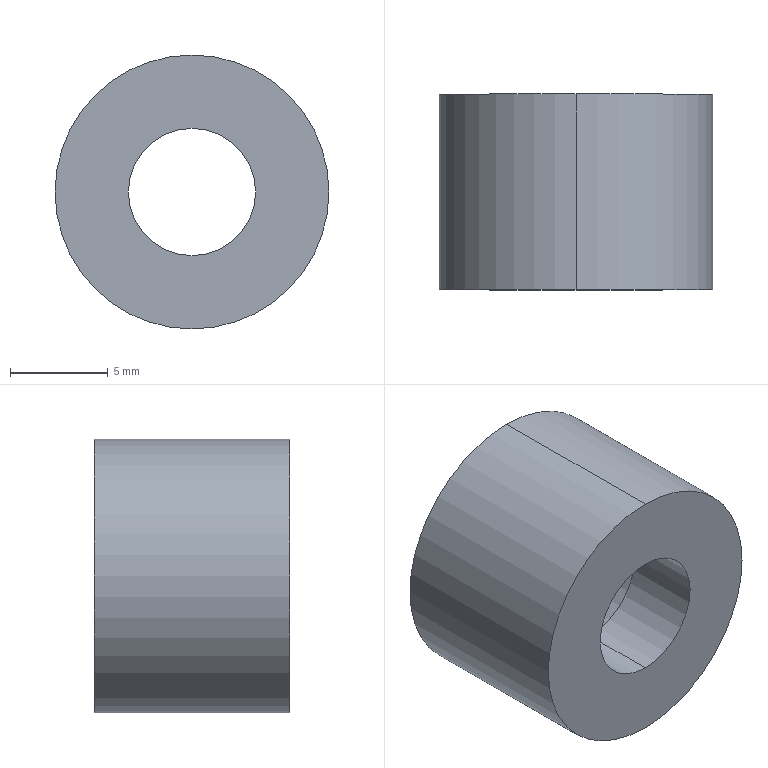Part | STEP file | OP10-160_seal pad (2nd air pass) | 1 solid | 9 faces | box 14 x 10 x 14 mm | volume 981.355 mm3 | cylinder 6 | plane 3 | commonest cylinder face diameters 6.5 x2 9.5 x2 14 x2
STEP:
#1=CARTESIAN_POINT('',(0.,0.,0.));
#2=DIRECTION('',(0.,0.,1.));
#3=DIRECTION('',(1.,0.,0.));
#4=AXIS2_PLACEMENT_3D('',#1,#2,#3);
#5=CARTESIAN_POINT('',(0.,4.,4.75));
#6=VERTEX_POINT('',#5);
#7=CARTESIAN_POINT('',(0.,10.,4.75));
#8=VERTEX_POINT('',#7);
#9=CARTESIAN_POINT('',(0.,4.,4.75));
#10=DIRECTION('',(0.,1.,0.));
#11=VECTOR('',#10,1.);
#12=LINE('',#9,#11);
#13=CARTESIAN_POINT('',(0.,4.,0.));
#14=DIRECTION('',(0.,1.,0.));
#15=DIRECTION('',(0.,0.,1.));
#16=AXIS2_PLACEMENT_3D('',#13,#14,#15);
#17=CYLINDRICAL_SURFACE('',#16,4.75);
#18=CARTESIAN_POINT('',(6.283,0.));
#19=DIRECTION('',(0.,1.));
#20=VECTOR('',#19,1.);
#21=LINE('',#18,#20);
#22=(GEOMETRIC_REPRESENTATION_CONTEXT(2)PARAMETRIC_REPRESENTATION_CONTEXT()REPRESENTATION_CONTEXT('',''));
#23=DEFINITIONAL_REPRESENTATION('',(#21),#22);
#24=PCURVE('',#17,#23);
#25=CARTESIAN_POINT('',(0.,4.,0.));
#26=DIRECTION('',(0.,1.,0.));
#27=DIRECTION('',(0.,0.,1.));
#28=AXIS2_PLACEMENT_3D('',#25,#26,#27);
#29=CYLINDRICAL_SURFACE('',#28,4.75);
#30=CARTESIAN_POINT('',(0.,0.));
#31=DIRECTION('',(0.,1.));
#32=VECTOR('',#31,1.);
#33=LINE('',#30,#32);
#34=(GEOMETRIC_REPRESENTATION_CONTEXT(2)PARAMETRIC_REPRESENTATION_CONTEXT()REPRESENTATION_CONTEXT('',''));
#35=DEFINITIONAL_REPRESENTATION('',(#33),#34);
#36=PCURVE('',#29,#35);
#37=SURFACE_CURVE('',#12,(#24,#36),.PCURVE_S1.);
#38=EDGE_CURVE('',#6,#8,#37,.T.);
#39=ORIENTED_EDGE('',*,*,#38,.T.);
#40=CARTESIAN_POINT('',(0.,10.,-4.75));
#41=VERTEX_POINT('',#40);
#42=CARTESIAN_POINT('',(0.,10.,0.));
#43=DIRECTION('',(0.,1.,0.));
#44=DIRECTION('',(0.,0.,1.));
#45=AXIS2_PLACEMENT_3D('',#42,#43,#44);
#46=CIRCLE('',#45,4.75);
#47=CARTESIAN_POINT('',(0.,6.));
#48=DIRECTION('',(1.,0.));
#49=VECTOR('',#48,1.);
#50=LINE('',#47,#49);
#51=(GEOMETRIC_REPRESENTATION_CONTEXT(2)PARAMETRIC_REPRESENTATION_CONTEXT()REPRESENTATION_CONTEXT('',''));
#52=DEFINITIONAL_REPRESENTATION('',(#50),#51);
#53=PCURVE('',#17,#52);
#54=CARTESIAN_POINT('',(0.,10.,0.));
#55=DIRECTION('',(0.,1.,0.));
#56=DIRECTION('',(0.,0.,1.));
#57=AXIS2_PLACEMENT_3D('',#54,#55,#56);
#58=PLANE('',#57);
#59=CARTESIAN_POINT('',(0.,0.));
#60=DIRECTION('',(1.,0.));
#61=AXIS2_PLACEMENT_2D('',#59,#60);
#62=CIRCLE('',#61,4.75);
#63=(GEOMETRIC_REPRESENTATION_CONTEXT(2)PARAMETRIC_REPRESENTATION_CONTEXT()REPRESENTATION_CONTEXT('',''));
#64=DEFINITIONAL_REPRESENTATION('',(#62),#63);
#65=PCURVE('',#58,#64);
#66=SURFACE_CURVE('',#46,(#53,#65),.PCURVE_S1.);
#67=EDGE_CURVE('',#41,#8,#66,.T.);
#68=ORIENTED_EDGE('',*,*,#67,.F.);
#69=CARTESIAN_POINT('',(0.,4.,-4.75));
#70=VERTEX_POINT('',#69);
#71=CARTESIAN_POINT('',(0.,4.,-4.75));
#72=DIRECTION('',(0.,1.,0.));
#73=VECTOR('',#72,1.);
#74=LINE('',#71,#73);
#75=CARTESIAN_POINT('',(3.142,0.));
#76=DIRECTION('',(0.,1.));
#77=VECTOR('',#76,1.);
#78=LINE('',#75,#77);
#79=(GEOMETRIC_REPRESENTATION_CONTEXT(2)PARAMETRIC_REPRESENTATION_CONTEXT()REPRESENTATION_CONTEXT('',''));
#80=DEFINITIONAL_REPRESENTATION('',(#78),#79);
#81=PCURVE('',#17,#80);
#82=CARTESIAN_POINT('',(3.142,0.));
#83=DIRECTION('',(0.,1.));
#84=VECTOR('',#83,1.);
#85=LINE('',#82,#84);
#86=(GEOMETRIC_REPRESENTATION_CONTEXT(2)PARAMETRIC_REPRESENTATION_CONTEXT()REPRESENTATION_CONTEXT('',''));
#87=DEFINITIONAL_REPRESENTATION('',(#85),#86);
#88=PCURVE('',#29,#87);
#89=SURFACE_CURVE('',#74,(#81,#88),.PCURVE_S1.);
#90=EDGE_CURVE('',#70,#41,#89,.T.);
#91=ORIENTED_EDGE('',*,*,#90,.F.);
#92=CARTESIAN_POINT('',(0.,4.,0.));
#93=DIRECTION('',(0.,1.,0.));
#94=DIRECTION('',(0.,0.,1.));
#95=AXIS2_PLACEMENT_3D('',#92,#93,#94);
#96=CIRCLE('',#95,4.75);
#97=CARTESIAN_POINT('',(0.,0.));
#98=DIRECTION('',(1.,0.));
#99=VECTOR('',#98,1.);
#100=LINE('',#97,#99);
#101=(GEOMETRIC_REPRESENTATION_CONTEXT(2)PARAMETRIC_REPRESENTATION_CONTEXT()REPRESENTATION_CONTEXT('',''));
#102=DEFINITIONAL_REPRESENTATION('',(#100),#101);
#103=PCURVE('',#17,#102);
#104=CARTESIAN_POINT('',(0.,4.,0.));
#105=DIRECTION('',(0.,1.,0.));
#106=DIRECTION('',(0.,0.,1.));
#107=AXIS2_PLACEMENT_3D('',#104,#105,#106);
#108=PLANE('',#107);
#109=CARTESIAN_POINT('',(0.,0.));
#110=DIRECTION('',(1.,0.));
#111=AXIS2_PLACEMENT_2D('',#109,#110);
#112=CIRCLE('',#111,4.75);
#113=(GEOMETRIC_REPRESENTATION_CONTEXT(2)PARAMETRIC_REPRESENTATION_CONTEXT()REPRESENTATION_CONTEXT('',''));
#114=DEFINITIONAL_REPRESENTATION('',(#112),#113);
#115=PCURVE('',#108,#114);
#116=SURFACE_CURVE('',#96,(#103,#115),.PCURVE_S1.);
#117=EDGE_CURVE('',#70,#6,#116,.T.);
#118=ORIENTED_EDGE('',*,*,#117,.T.);
#119=EDGE_LOOP('',(#39,#68,#91,#118));
#120=FACE_BOUND('',#119,.F.);
#121=ADVANCED_FACE('',(#120),#17,.F.);
#122=CARTESIAN_POINT('',(0.,10.,7.));
#123=VERTEX_POINT('',#122);
#124=CARTESIAN_POINT('',(0.,10.,-7.));
#125=VERTEX_POINT('',#124);
#126=CARTESIAN_POINT('',(0.,10.,0.));
#127=DIRECTION('',(0.,1.,0.));
#128=DIRECTION('',(0.,0.,1.));
#129=AXIS2_PLACEMENT_3D('',#126,#127,#128);
#130=CIRCLE('',#129,7.);
#131=CARTESIAN_POINT('',(0.,10.,0.));
#132=DIRECTION('',(0.,-1.,0.));
#133=DIRECTION('',(0.,0.,-1.));
#134=AXIS2_PLACEMENT_3D('',#131,#132,#133);
#135=CYLINDRICAL_SURFACE('',#134,7.);
#136=CARTESIAN_POINT('',(3.142,0.));
#137=DIRECTION('',(-1.,0.));
#138=VECTOR('',#137,1.);
#139=LINE('',#136,#138);
#140=(GEOMETRIC_REPRESENTATION_CONTEXT(2)PARAMETRIC_REPRESENTATION_CONTEXT()REPRESENTATION_CONTEXT('',''));
#141=DEFINITIONAL_REPRESENTATION('',(#139),#140);
#142=PCURVE('',#135,#141);
#143=CARTESIAN_POINT('',(0.,0.));
#144=DIRECTION('',(1.,0.));
#145=AXIS2_PLACEMENT_2D('',#143,#144);
#146=CIRCLE('',#145,7.);
#147=(GEOMETRIC_REPRESENTATION_CONTEXT(2)PARAMETRIC_REPRESENTATION_CONTEXT()REPRESENTATION_CONTEXT('',''));
#148=DEFINITIONAL_REPRESENTATION('',(#146),#147);
#149=PCURVE('',#58,#148);
#150=SURFACE_CURVE('',#130,(#142,#149),.PCURVE_S1.);
#151=EDGE_CURVE('',#123,#125,#150,.T.);
#152=ORIENTED_EDGE('',*,*,#151,.F.);
#153=CARTESIAN_POINT('',(0.,0.,7.));
#154=VERTEX_POINT('',#153);
#155=CARTESIAN_POINT('',(0.,10.,7.));
#156=DIRECTION('',(0.,-1.,0.));
#157=VECTOR('',#156,1.);
#158=LINE('',#155,#157);
#159=CARTESIAN_POINT('',(3.142,0.));
#160=DIRECTION('',(0.,1.));
#161=VECTOR('',#160,1.);
#162=LINE('',#159,#161);
#163=(GEOMETRIC_REPRESENTATION_CONTEXT(2)PARAMETRIC_REPRESENTATION_CONTEXT()REPRESENTATION_CONTEXT('',''));
#164=DEFINITIONAL_REPRESENTATION('',(#162),#163);
#165=PCURVE('',#135,#164);
#166=CARTESIAN_POINT('',(0.,10.,0.));
#167=DIRECTION('',(0.,-1.,0.));
#168=DIRECTION('',(0.,0.,-1.));
#169=AXIS2_PLACEMENT_3D('',#166,#167,#168);
#170=CYLINDRICAL_SURFACE('',#169,7.);
#171=CARTESIAN_POINT('',(3.142,0.));
#172=DIRECTION('',(0.,1.));
#173=VECTOR('',#172,1.);
#174=LINE('',#171,#173);
#175=(GEOMETRIC_REPRESENTATION_CONTEXT(2)PARAMETRIC_REPRESENTATION_CONTEXT()REPRESENTATION_CONTEXT('',''));
#176=DEFINITIONAL_REPRESENTATION('',(#174),#175);
#177=PCURVE('',#170,#176);
#178=SURFACE_CURVE('',#158,(#165,#177),.PCURVE_S1.);
#179=EDGE_CURVE('',#123,#154,#178,.T.);
#180=ORIENTED_EDGE('',*,*,#179,.T.);
#181=CARTESIAN_POINT('',(0.,0.,-7.));
#182=VERTEX_POINT('',#181);
#183=CARTESIAN_POINT('',(0.,0.,0.));
#184=DIRECTION('',(0.,1.,0.));
#185=DIRECTION('',(0.,0.,1.));
#186=AXIS2_PLACEMENT_3D('',#183,#184,#185);
#187=CIRCLE('',#186,7.);
#188=CARTESIAN_POINT('',(3.142,10.));
#189=DIRECTION('',(-1.,0.));
#190=VECTOR('',#189,1.);
#191=LINE('',#188,#190);
#192=(GEOMETRIC_REPRESENTATION_CONTEXT(2)PARAMETRIC_REPRESENTATION_CONTEXT()REPRESENTATION_CONTEXT('',''));
#193=DEFINITIONAL_REPRESENTATION('',(#191),#192);
#194=PCURVE('',#135,#193);
#195=CARTESIAN_POINT('',(0.,0.,0.));
#196=DIRECTION('',(0.,1.,0.));
#197=DIRECTION('',(0.,0.,1.));
#198=AXIS2_PLACEMENT_3D('',#195,#196,#197);
#199=PLANE('',#198);
#200=CARTESIAN_POINT('',(0.,0.));
#201=DIRECTION('',(1.,0.));
#202=AXIS2_PLACEMENT_2D('',#200,#201);
#203=CIRCLE('',#202,7.);
#204=(GEOMETRIC_REPRESENTATION_CONTEXT(2)PARAMETRIC_REPRESENTATION_CONTEXT()REPRESENTATION_CONTEXT('',''));
#205=DEFINITIONAL_REPRESENTATION('',(#203),#204);
#206=PCURVE('',#199,#205);
#207=SURFACE_CURVE('',#187,(#194,#206),.PCURVE_S1.);
#208=EDGE_CURVE('',#154,#182,#207,.T.);
#209=ORIENTED_EDGE('',*,*,#208,.T.);
#210=CARTESIAN_POINT('',(0.,10.,-7.));
#211=DIRECTION('',(0.,-1.,0.));
#212=VECTOR('',#211,1.);
#213=LINE('',#210,#212);
#214=CARTESIAN_POINT('',(0.,0.));
#215=DIRECTION('',(0.,1.));
#216=VECTOR('',#215,1.);
#217=LINE('',#214,#216);
#218=(GEOMETRIC_REPRESENTATION_CONTEXT(2)PARAMETRIC_REPRESENTATION_CONTEXT()REPRESENTATION_CONTEXT('',''));
#219=DEFINITIONAL_REPRESENTATION('',(#217),#218);
#220=PCURVE('',#135,#219);
#221=CARTESIAN_POINT('',(6.283,0.));
#222=DIRECTION('',(0.,1.));
#223=VECTOR('',#222,1.);
#224=LINE('',#221,#223);
#225=(GEOMETRIC_REPRESENTATION_CONTEXT(2)PARAMETRIC_REPRESENTATION_CONTEXT()REPRESENTATION_CONTEXT('',''));
#226=DEFINITIONAL_REPRESENTATION('',(#224),#225);
#227=PCURVE('',#170,#226);
#228=SURFACE_CURVE('',#213,(#220,#227),.PCURVE_S1.);
#229=EDGE_CURVE('',#125,#182,#228,.T.);
#230=ORIENTED_EDGE('',*,*,#229,.F.);
#231=EDGE_LOOP('',(#152,#180,#209,#230));
#232=FACE_BOUND('',#231,.T.);
#233=ADVANCED_FACE('',(#232),#135,.T.);
#234=CARTESIAN_POINT('',(0.,0.,3.25));
#235=VERTEX_POINT('',#234);
#236=CARTESIAN_POINT('',(0.,4.,3.25));
#237=VERTEX_POINT('',#236);
#238=CARTESIAN_POINT('',(0.,10.,3.25));
#239=DIRECTION('',(0.,1.,0.));
#240=VECTOR('',#239,1.);
#241=LINE('',#238,#240);
#242=CARTESIAN_POINT('',(0.,10.,0.));
#243=DIRECTION('',(0.,1.,0.));
#244=DIRECTION('',(0.,0.,1.));
#245=AXIS2_PLACEMENT_3D('',#242,#243,#244);
#246=CYLINDRICAL_SURFACE('',#245,3.25);
#247=CARTESIAN_POINT('',(6.283,0.));
#248=DIRECTION('',(0.,1.));
#249=VECTOR('',#248,1.);
#250=LINE('',#247,#249);
#251=(GEOMETRIC_REPRESENTATION_CONTEXT(2)PARAMETRIC_REPRESENTATION_CONTEXT()REPRESENTATION_CONTEXT('',''));
#252=DEFINITIONAL_REPRESENTATION('',(#250),#251);
#253=PCURVE('',#246,#252);
#254=CARTESIAN_POINT('',(0.,10.,0.));
#255=DIRECTION('',(0.,1.,0.));
#256=DIRECTION('',(0.,0.,1.));
#257=AXIS2_PLACEMENT_3D('',#254,#255,#256);
#258=CYLINDRICAL_SURFACE('',#257,3.25);
#259=CARTESIAN_POINT('',(0.,0.));
#260=DIRECTION('',(0.,1.));
#261=VECTOR('',#260,1.);
#262=LINE('',#259,#261);
#263=(GEOMETRIC_REPRESENTATION_CONTEXT(2)PARAMETRIC_REPRESENTATION_CONTEXT()REPRESENTATION_CONTEXT('',''));
#264=DEFINITIONAL_REPRESENTATION('',(#262),#263);
#265=PCURVE('',#258,#264);
#266=SURFACE_CURVE('',#241,(#253,#265),.PCURVE_S1.);
#267=EDGE_CURVE('',#235,#237,#266,.T.);
#268=ORIENTED_EDGE('',*,*,#267,.T.);
#269=CARTESIAN_POINT('',(0.,4.,-3.25));
#270=VERTEX_POINT('',#269);
#271=CARTESIAN_POINT('',(0.,4.,0.));
#272=DIRECTION('',(0.,-1.,0.));
#273=DIRECTION('',(0.,0.,1.));
#274=AXIS2_PLACEMENT_3D('',#271,#272,#273);
#275=CIRCLE('',#274,3.25);
#276=CARTESIAN_POINT('',(6.283,-6.));
#277=DIRECTION('',(-1.,0.));
#278=VECTOR('',#277,1.);
#279=LINE('',#276,#278);
#280=(GEOMETRIC_REPRESENTATION_CONTEXT(2)PARAMETRIC_REPRESENTATION_CONTEXT()REPRESENTATION_CONTEXT('',''));
#281=DEFINITIONAL_REPRESENTATION('',(#279),#280);
#282=PCURVE('',#246,#281);
#283=CARTESIAN_POINT('',(3.25,0.));
#284=CARTESIAN_POINT('',(3.25,-5.629));
#285=CARTESIAN_POINT('',(-1.625,-2.815));
#286=CARTESIAN_POINT('',(-6.5,0.));
#287=CARTESIAN_POINT('',(-1.625,2.815));
#288=CARTESIAN_POINT('',(3.25,5.629));
#289=CARTESIAN_POINT('',(3.25,0.));
#290=(BOUNDED_CURVE()B_SPLINE_CURVE(2,(#283,#284,#285,#286,#287,#288,#289),.UNSPECIFIED.,.T.,.F.)B_SPLINE_CURVE_WITH_KNOTS((1,2,2,2,2,1),(-2.094,0.,2.094,4.189,6.283,8.378),.UNSPECIFIED.)CURVE()GEOMETRIC_REPRESENTATION_ITEM()RATIONAL_B_SPLINE_CURVE((1.,0.5,1.,0.5,1.,0.5,1.))REPRESENTATION_ITEM(''));
#291=(GEOMETRIC_REPRESENTATION_CONTEXT(2)PARAMETRIC_REPRESENTATION_CONTEXT()REPRESENTATION_CONTEXT('',''));
#292=DEFINITIONAL_REPRESENTATION('',(#290),#291);
#293=PCURVE('',#108,#292);
#294=SURFACE_CURVE('',#275,(#282,#293),.PCURVE_S1.);
#295=EDGE_CURVE('',#237,#270,#294,.T.);
#296=ORIENTED_EDGE('',*,*,#295,.T.);
#297=CARTESIAN_POINT('',(0.,0.,-3.25));
#298=VERTEX_POINT('',#297);
#299=CARTESIAN_POINT('',(0.,10.,-3.25));
#300=DIRECTION('',(0.,1.,0.));
#301=VECTOR('',#300,1.);
#302=LINE('',#299,#301);
#303=CARTESIAN_POINT('',(3.142,0.));
#304=DIRECTION('',(0.,1.));
#305=VECTOR('',#304,1.);
#306=LINE('',#303,#305);
#307=(GEOMETRIC_REPRESENTATION_CONTEXT(2)PARAMETRIC_REPRESENTATION_CONTEXT()REPRESENTATION_CONTEXT('',''));
#308=DEFINITIONAL_REPRESENTATION('',(#306),#307);
#309=PCURVE('',#246,#308);
#310=CARTESIAN_POINT('',(3.142,0.));
#311=DIRECTION('',(0.,1.));
#312=VECTOR('',#311,1.);
#313=LINE('',#310,#312);
#314=(GEOMETRIC_REPRESENTATION_CONTEXT(2)PARAMETRIC_REPRESENTATION_CONTEXT()REPRESENTATION_CONTEXT('',''));
#315=DEFINITIONAL_REPRESENTATION('',(#313),#314);
#316=PCURVE('',#258,#315);
#317=SURFACE_CURVE('',#302,(#309,#316),.PCURVE_S1.);
#318=EDGE_CURVE('',#298,#270,#317,.T.);
#319=ORIENTED_EDGE('',*,*,#318,.F.);
#320=CARTESIAN_POINT('',(0.,0.,0.));
#321=DIRECTION('',(0.,1.,0.));
#322=DIRECTION('',(0.,0.,1.));
#323=AXIS2_PLACEMENT_3D('',#320,#321,#322);
#324=CIRCLE('',#323,3.25);
#325=CARTESIAN_POINT('',(0.,-10.));
#326=DIRECTION('',(1.,0.));
#327=VECTOR('',#326,1.);
#328=LINE('',#325,#327);
#329=(GEOMETRIC_REPRESENTATION_CONTEXT(2)PARAMETRIC_REPRESENTATION_CONTEXT()REPRESENTATION_CONTEXT('',''));
#330=DEFINITIONAL_REPRESENTATION('',(#328),#329);
#331=PCURVE('',#246,#330);
#332=CARTESIAN_POINT('',(0.,0.));
#333=DIRECTION('',(1.,0.));
#334=AXIS2_PLACEMENT_2D('',#332,#333);
#335=CIRCLE('',#334,3.25);
#336=(GEOMETRIC_REPRESENTATION_CONTEXT(2)PARAMETRIC_REPRESENTATION_CONTEXT()REPRESENTATION_CONTEXT('',''));
#337=DEFINITIONAL_REPRESENTATION('',(#335),#336);
#338=PCURVE('',#199,#337);
#339=SURFACE_CURVE('',#324,(#331,#338),.PCURVE_S1.);
#340=EDGE_CURVE('',#298,#235,#339,.T.);
#341=ORIENTED_EDGE('',*,*,#340,.T.);
#342=EDGE_LOOP('',(#268,#296,#319,#341));
#343=FACE_BOUND('',#342,.F.);
#344=ADVANCED_FACE('',(#343),#246,.F.);
#345=CARTESIAN_POINT('',(0.,4.,0.));
#346=DIRECTION('',(0.,-1.,0.));
#347=DIRECTION('',(0.,0.,1.));
#348=AXIS2_PLACEMENT_3D('',#345,#346,#347);
#349=CIRCLE('',#348,3.25);
#350=CARTESIAN_POINT('',(6.283,-6.));
#351=DIRECTION('',(-1.,0.));
#352=VECTOR('',#351,1.);
#353=LINE('',#350,#352);
#354=(GEOMETRIC_REPRESENTATION_CONTEXT(2)PARAMETRIC_REPRESENTATION_CONTEXT()REPRESENTATION_CONTEXT('',''));
#355=DEFINITIONAL_REPRESENTATION('',(#353),#354);
#356=PCURVE('',#258,#355);
#357=CARTESIAN_POINT('',(3.25,0.));
#358=CARTESIAN_POINT('',(3.25,-5.629));
#359=CARTESIAN_POINT('',(-1.625,-2.815));
#360=CARTESIAN_POINT('',(-6.5,0.));
#361=CARTESIAN_POINT('',(-1.625,2.815));
#362=CARTESIAN_POINT('',(3.25,5.629));
#363=CARTESIAN_POINT('',(3.25,0.));
#364=(BOUNDED_CURVE()B_SPLINE_CURVE(2,(#357,#358,#359,#360,#361,#362,#363),.UNSPECIFIED.,.T.,.F.)B_SPLINE_CURVE_WITH_KNOTS((1,2,2,2,2,1),(-2.094,0.,2.094,4.189,6.283,8.378),.UNSPECIFIED.)CURVE()GEOMETRIC_REPRESENTATION_ITEM()RATIONAL_B_SPLINE_CURVE((1.,0.5,1.,0.5,1.,0.5,1.))REPRESENTATION_ITEM(''));
#365=(GEOMETRIC_REPRESENTATION_CONTEXT(2)PARAMETRIC_REPRESENTATION_CONTEXT()REPRESENTATION_CONTEXT('',''));
#366=DEFINITIONAL_REPRESENTATION('',(#364),#365);
#367=PCURVE('',#108,#366);
#368=SURFACE_CURVE('',#349,(#356,#367),.PCURVE_S1.);
#369=EDGE_CURVE('',#270,#237,#368,.T.);
#370=ORIENTED_EDGE('',*,*,#369,.T.);
#371=ORIENTED_EDGE('',*,*,#267,.F.);
#372=CARTESIAN_POINT('',(0.,0.,0.));
#373=DIRECTION('',(0.,1.,0.));
#374=DIRECTION('',(0.,0.,1.));
#375=AXIS2_PLACEMENT_3D('',#372,#373,#374);
#376=CIRCLE('',#375,3.25);
#377=CARTESIAN_POINT('',(0.,-10.));
#378=DIRECTION('',(1.,0.));
#379=VECTOR('',#378,1.);
#380=LINE('',#377,#379);
#381=(GEOMETRIC_REPRESENTATION_CONTEXT(2)PARAMETRIC_REPRESENTATION_CONTEXT()REPRESENTATION_CONTEXT('',''));
#382=DEFINITIONAL_REPRESENTATION('',(#380),#381);
#383=PCURVE('',#258,#382);
#384=CARTESIAN_POINT('',(0.,0.));
#385=DIRECTION('',(1.,0.));
#386=AXIS2_PLACEMENT_2D('',#384,#385);
#387=CIRCLE('',#386,3.25);
#388=(GEOMETRIC_REPRESENTATION_CONTEXT(2)PARAMETRIC_REPRESENTATION_CONTEXT()REPRESENTATION_CONTEXT('',''));
#389=DEFINITIONAL_REPRESENTATION('',(#387),#388);
#390=PCURVE('',#199,#389);
#391=SURFACE_CURVE('',#376,(#383,#390),.PCURVE_S1.);
#392=EDGE_CURVE('',#235,#298,#391,.T.);
#393=ORIENTED_EDGE('',*,*,#392,.T.);
#394=ORIENTED_EDGE('',*,*,#318,.T.);
#395=EDGE_LOOP('',(#370,#371,#393,#394));
#396=FACE_BOUND('',#395,.F.);
#397=ADVANCED_FACE('',(#396),#258,.F.);
#398=ORIENTED_EDGE('',*,*,#179,.F.);
#399=CARTESIAN_POINT('',(0.,10.,0.));
#400=DIRECTION('',(0.,1.,0.));
#401=DIRECTION('',(0.,0.,1.));
#402=AXIS2_PLACEMENT_3D('',#399,#400,#401);
#403=CIRCLE('',#402,7.);
#404=CARTESIAN_POINT('',(9.425,0.));
#405=DIRECTION('',(-1.,0.));
#406=VECTOR('',#405,1.);
#407=LINE('',#404,#406);
#408=(GEOMETRIC_REPRESENTATION_CONTEXT(2)PARAMETRIC_REPRESENTATION_CONTEXT()REPRESENTATION_CONTEXT('',''));
#409=DEFINITIONAL_REPRESENTATION('',(#407),#408);
#410=PCURVE('',#170,#409);
#411=CARTESIAN_POINT('',(0.,0.));
#412=DIRECTION('',(1.,0.));
#413=AXIS2_PLACEMENT_2D('',#411,#412);
#414=CIRCLE('',#413,7.);
#415=(GEOMETRIC_REPRESENTATION_CONTEXT(2)PARAMETRIC_REPRESENTATION_CONTEXT()REPRESENTATION_CONTEXT('',''));
#416=DEFINITIONAL_REPRESENTATION('',(#414),#415);
#417=PCURVE('',#58,#416);
#418=SURFACE_CURVE('',#403,(#410,#417),.PCURVE_S1.);
#419=EDGE_CURVE('',#125,#123,#418,.T.);
#420=ORIENTED_EDGE('',*,*,#419,.F.);
#421=ORIENTED_EDGE('',*,*,#229,.T.);
#422=CARTESIAN_POINT('',(0.,0.,0.));
#423=DIRECTION('',(0.,1.,0.));
#424=DIRECTION('',(0.,0.,1.));
#425=AXIS2_PLACEMENT_3D('',#422,#423,#424);
#426=CIRCLE('',#425,7.);
#427=CARTESIAN_POINT('',(9.425,10.));
#428=DIRECTION('',(-1.,0.));
#429=VECTOR('',#428,1.);
#430=LINE('',#427,#429);
#431=(GEOMETRIC_REPRESENTATION_CONTEXT(2)PARAMETRIC_REPRESENTATION_CONTEXT()REPRESENTATION_CONTEXT('',''));
#432=DEFINITIONAL_REPRESENTATION('',(#430),#431);
#433=PCURVE('',#170,#432);
#434=CARTESIAN_POINT('',(0.,0.));
#435=DIRECTION('',(1.,0.));
#436=AXIS2_PLACEMENT_2D('',#434,#435);
#437=CIRCLE('',#436,7.);
#438=(GEOMETRIC_REPRESENTATION_CONTEXT(2)PARAMETRIC_REPRESENTATION_CONTEXT()REPRESENTATION_CONTEXT('',''));
#439=DEFINITIONAL_REPRESENTATION('',(#437),#438);
#440=PCURVE('',#199,#439);
#441=SURFACE_CURVE('',#426,(#433,#440),.PCURVE_S1.);
#442=EDGE_CURVE('',#182,#154,#441,.T.);
#443=ORIENTED_EDGE('',*,*,#442,.T.);
#444=EDGE_LOOP('',(#398,#420,#421,#443));
#445=FACE_BOUND('',#444,.T.);
#446=ADVANCED_FACE('',(#445),#170,.T.);
#447=CARTESIAN_POINT('',(0.,10.,0.));
#448=DIRECTION('',(0.,1.,0.));
#449=DIRECTION('',(0.,0.,1.));
#450=AXIS2_PLACEMENT_3D('',#447,#448,#449);
#451=CIRCLE('',#450,4.75);
#452=CARTESIAN_POINT('',(0.,0.));
#453=DIRECTION('',(1.,0.));
#454=AXIS2_PLACEMENT_2D('',#452,#453);
#455=CIRCLE('',#454,4.75);
#456=(GEOMETRIC_REPRESENTATION_CONTEXT(2)PARAMETRIC_REPRESENTATION_CONTEXT()REPRESENTATION_CONTEXT('',''));
#457=DEFINITIONAL_REPRESENTATION('',(#455),#456);
#458=PCURVE('',#58,#457);
#459=CARTESIAN_POINT('',(0.,6.));
#460=DIRECTION('',(1.,0.));
#461=VECTOR('',#460,1.);
#462=LINE('',#459,#461);
#463=(GEOMETRIC_REPRESENTATION_CONTEXT(2)PARAMETRIC_REPRESENTATION_CONTEXT()REPRESENTATION_CONTEXT('',''));
#464=DEFINITIONAL_REPRESENTATION('',(#462),#463);
#465=PCURVE('',#29,#464);
#466=SURFACE_CURVE('',#451,(#458,#465),.PCURVE_S1.);
#467=EDGE_CURVE('',#8,#41,#466,.T.);
#468=ORIENTED_EDGE('',*,*,#467,.F.);
#469=ORIENTED_EDGE('',*,*,#67,.F.);
#470=EDGE_LOOP('',(#468,#469));
#471=FACE_BOUND('',#470,.T.);
#472=ORIENTED_EDGE('',*,*,#419,.T.);
#473=ORIENTED_EDGE('',*,*,#151,.T.);
#474=EDGE_LOOP('',(#472,#473));
#475=FACE_BOUND('',#474,.T.);
#476=ADVANCED_FACE('',(#471,#475),#58,.T.);
#477=ORIENTED_EDGE('',*,*,#392,.T.);
#478=ORIENTED_EDGE('',*,*,#340,.T.);
#479=EDGE_LOOP('',(#477,#478));
#480=FACE_BOUND('',#479,.T.);
#481=ORIENTED_EDGE('',*,*,#442,.F.);
#482=ORIENTED_EDGE('',*,*,#208,.F.);
#483=EDGE_LOOP('',(#481,#482));
#484=FACE_BOUND('',#483,.T.);
#485=ADVANCED_FACE('',(#480,#484),#199,.F.);
#486=CARTESIAN_POINT('',(0.,4.,0.));
#487=DIRECTION('',(0.,1.,0.));
#488=DIRECTION('',(0.,0.,1.));
#489=AXIS2_PLACEMENT_3D('',#486,#487,#488);
#490=CIRCLE('',#489,4.75);
#491=CARTESIAN_POINT('',(0.,0.));
#492=DIRECTION('',(1.,0.));
#493=AXIS2_PLACEMENT_2D('',#491,#492);
#494=CIRCLE('',#493,4.75);
#495=(GEOMETRIC_REPRESENTATION_CONTEXT(2)PARAMETRIC_REPRESENTATION_CONTEXT()REPRESENTATION_CONTEXT('',''));
#496=DEFINITIONAL_REPRESENTATION('',(#494),#495);
#497=PCURVE('',#108,#496);
#498=CARTESIAN_POINT('',(0.,0.));
#499=DIRECTION('',(1.,0.));
#500=VECTOR('',#499,1.);
#501=LINE('',#498,#500);
#502=(GEOMETRIC_REPRESENTATION_CONTEXT(2)PARAMETRIC_REPRESENTATION_CONTEXT()REPRESENTATION_CONTEXT('',''));
#503=DEFINITIONAL_REPRESENTATION('',(#501),#502);
#504=PCURVE('',#29,#503);
#505=SURFACE_CURVE('',#490,(#497,#504),.PCURVE_S1.);
#506=EDGE_CURVE('',#6,#70,#505,.T.);
#507=ORIENTED_EDGE('',*,*,#506,.T.);
#508=ORIENTED_EDGE('',*,*,#117,.T.);
#509=EDGE_LOOP('',(#507,#508));
#510=FACE_BOUND('',#509,.T.);
#511=ORIENTED_EDGE('',*,*,#295,.T.);
#512=ORIENTED_EDGE('',*,*,#369,.T.);
#513=EDGE_LOOP('',(#511,#512));
#514=FACE_BOUND('',#513,.T.);
#515=ADVANCED_FACE('',(#510,#514),#108,.T.);
#516=ORIENTED_EDGE('',*,*,#467,.F.);
#517=ORIENTED_EDGE('',*,*,#38,.F.);
#518=ORIENTED_EDGE('',*,*,#506,.T.);
#519=ORIENTED_EDGE('',*,*,#90,.T.);
#520=EDGE_LOOP('',(#516,#517,#518,#519));
#521=FACE_BOUND('',#520,.F.);
#522=ADVANCED_FACE('',(#521),#29,.F.);
#523=CLOSED_SHELL('',(#121,#233,#344,#397,#446,#476,#485,#515,#522));
#524=MANIFOLD_SOLID_BREP('',#523);
#525=(LENGTH_UNIT()NAMED_UNIT(*)SI_UNIT(.MILLI.,.METRE.));
#526=UNCERTAINTY_MEASURE_WITH_UNIT(LENGTH_MEASURE(0.0000001),#525,'','');
#527=(NAMED_UNIT(*)PLANE_ANGLE_UNIT()SI_UNIT($,.RADIAN.));
#528=(NAMED_UNIT(*)SI_UNIT($,.STERADIAN.)SOLID_ANGLE_UNIT());
#529=(GEOMETRIC_REPRESENTATION_CONTEXT(3)GLOBAL_UNCERTAINTY_ASSIGNED_CONTEXT((#526))GLOBAL_UNIT_ASSIGNED_CONTEXT((#525,#527,#528))REPRESENTATION_CONTEXT('',''));
#530=ADVANCED_BREP_SHAPE_REPRESENTATION('',(#4,#524),#529);